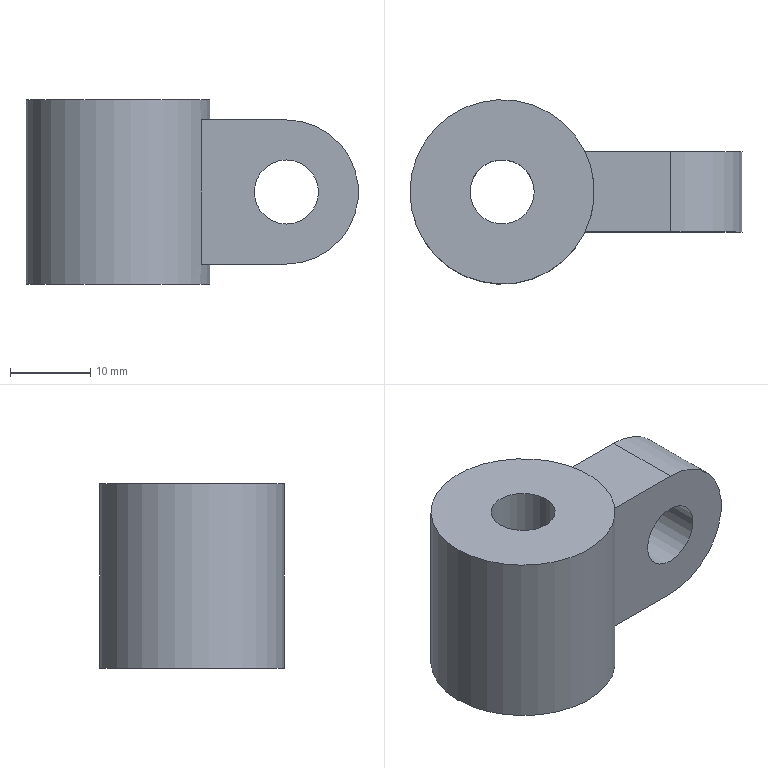Part | STEP file | 1 solid | 10 faces | box 41.5 x 23 x 23 mm | volume 10947 mm3 | plane 6 | cylinder 4 | commonest cylinder face diameters 8 x2 18 x1 23 x1
STEP:
#1=CARTESIAN_POINT('',(0.,0.,0.));
#2=DIRECTION('',(0.,0.,1.));
#3=DIRECTION('',(1.,0.,0.));
#4=AXIS2_PLACEMENT_3D('',#1,#2,#3);
#5=CARTESIAN_POINT('',(-11.5,0.,11.5));
#6=VERTEX_POINT('',#5);
#7=CARTESIAN_POINT('',(0.,0.,11.5));
#8=DIRECTION('',(0.,0.,-1.));
#9=DIRECTION('',(-1.,0.,0.));
#10=AXIS2_PLACEMENT_3D('',#7,#8,#9);
#11=CIRCLE('',#10,11.5);
#12=CARTESIAN_POINT('',(0.,0.,11.5));
#13=DIRECTION('',(0.,0.,-1.));
#14=DIRECTION('',(-1.,0.,0.));
#15=AXIS2_PLACEMENT_3D('',#12,#13,#14);
#16=CYLINDRICAL_SURFACE('',#15,11.5);
#17=CARTESIAN_POINT('',(0.,0.));
#18=DIRECTION('',(1.,0.));
#19=VECTOR('',#18,1.);
#20=LINE('',#17,#19);
#21=(GEOMETRIC_REPRESENTATION_CONTEXT(2)PARAMETRIC_REPRESENTATION_CONTEXT()REPRESENTATION_CONTEXT('',''));
#22=DEFINITIONAL_REPRESENTATION('',(#20),#21);
#23=PCURVE('',#16,#22);
#24=CARTESIAN_POINT('',(0.,0.,11.5));
#25=DIRECTION('',(0.,0.,1.));
#26=DIRECTION('',(1.,0.,0.));
#27=AXIS2_PLACEMENT_3D('',#24,#25,#26);
#28=PLANE('',#27);
#29=CARTESIAN_POINT('',(-11.5,0.));
#30=CARTESIAN_POINT('',(-11.5,19.919));
#31=CARTESIAN_POINT('',(5.75,9.959));
#32=CARTESIAN_POINT('',(23.,0.));
#33=CARTESIAN_POINT('',(5.75,-9.959));
#34=CARTESIAN_POINT('',(-11.5,-19.919));
#35=CARTESIAN_POINT('',(-11.5,0.));
#36=(BOUNDED_CURVE()B_SPLINE_CURVE(2,(#29,#30,#31,#32,#33,#34,#35),.UNSPECIFIED.,.T.,.F.)B_SPLINE_CURVE_WITH_KNOTS((1,2,2,2,2,1),(-2.094,0.,2.094,4.189,6.283,8.378),.UNSPECIFIED.)CURVE()GEOMETRIC_REPRESENTATION_ITEM()RATIONAL_B_SPLINE_CURVE((1.,0.5,1.,0.5,1.,0.5,1.))REPRESENTATION_ITEM(''));
#37=(GEOMETRIC_REPRESENTATION_CONTEXT(2)PARAMETRIC_REPRESENTATION_CONTEXT()REPRESENTATION_CONTEXT('',''));
#38=DEFINITIONAL_REPRESENTATION('',(#36),#37);
#39=PCURVE('',#28,#38);
#40=SURFACE_CURVE('',#11,(#23,#39),.PCURVE_S1.);
#41=EDGE_CURVE('',#6,#6,#40,.T.);
#42=ORIENTED_EDGE('',*,*,#41,.T.);
#43=CARTESIAN_POINT('',(-11.5,0.,-11.5));
#44=VERTEX_POINT('',#43);
#45=CARTESIAN_POINT('',(-11.5,0.,11.5));
#46=CARTESIAN_POINT('',(-11.5,0.,-11.5));
#47=B_SPLINE_CURVE_WITH_KNOTS('',1,(#45,#46),.UNSPECIFIED.,.F.,.F.,(2,2),(0.,23.),.PIECEWISE_BEZIER_KNOTS.);
#48=CARTESIAN_POINT('',(6.283,0.));
#49=DIRECTION('',(0.,1.));
#50=VECTOR('',#49,1.);
#51=LINE('',#48,#50);
#52=(GEOMETRIC_REPRESENTATION_CONTEXT(2)PARAMETRIC_REPRESENTATION_CONTEXT()REPRESENTATION_CONTEXT('',''));
#53=DEFINITIONAL_REPRESENTATION('',(#51),#52);
#54=PCURVE('',#16,#53);
#55=CARTESIAN_POINT('',(0.,0.));
#56=DIRECTION('',(0.,1.));
#57=VECTOR('',#56,1.);
#58=LINE('',#55,#57);
#59=(GEOMETRIC_REPRESENTATION_CONTEXT(2)PARAMETRIC_REPRESENTATION_CONTEXT()REPRESENTATION_CONTEXT('',''));
#60=DEFINITIONAL_REPRESENTATION('',(#58),#59);
#61=PCURVE('',#16,#60);
#62=SEAM_CURVE('',#47,(#54,#61),.PCURVE_S1.);
#63=EDGE_CURVE('',#6,#44,#62,.T.);
#64=ORIENTED_EDGE('',*,*,#63,.T.);
#65=CARTESIAN_POINT('',(0.,0.,-11.5));
#66=DIRECTION('',(0.,0.,1.));
#67=DIRECTION('',(-1.,0.,0.));
#68=AXIS2_PLACEMENT_3D('',#65,#66,#67);
#69=CIRCLE('',#68,11.5);
#70=CARTESIAN_POINT('',(6.283,23.));
#71=DIRECTION('',(-1.,0.));
#72=VECTOR('',#71,1.);
#73=LINE('',#70,#72);
#74=(GEOMETRIC_REPRESENTATION_CONTEXT(2)PARAMETRIC_REPRESENTATION_CONTEXT()REPRESENTATION_CONTEXT('',''));
#75=DEFINITIONAL_REPRESENTATION('',(#73),#74);
#76=PCURVE('',#16,#75);
#77=CARTESIAN_POINT('',(0.,0.,-11.5));
#78=DIRECTION('',(0.,0.,1.));
#79=DIRECTION('',(1.,0.,0.));
#80=AXIS2_PLACEMENT_3D('',#77,#78,#79);
#81=PLANE('',#80);
#82=CARTESIAN_POINT('',(0.,0.));
#83=DIRECTION('',(-1.,0.));
#84=AXIS2_PLACEMENT_2D('',#82,#83);
#85=CIRCLE('',#84,11.5);
#86=(GEOMETRIC_REPRESENTATION_CONTEXT(2)PARAMETRIC_REPRESENTATION_CONTEXT()REPRESENTATION_CONTEXT('',''));
#87=DEFINITIONAL_REPRESENTATION('',(#85),#86);
#88=PCURVE('',#81,#87);
#89=SURFACE_CURVE('',#69,(#76,#88),.PCURVE_S1.);
#90=EDGE_CURVE('',#44,#44,#89,.T.);
#91=ORIENTED_EDGE('',*,*,#90,.T.);
#92=ORIENTED_EDGE('',*,*,#63,.F.);
#93=EDGE_LOOP('',(#42,#64,#91,#92));
#94=FACE_BOUND('',#93,.T.);
#95=CARTESIAN_POINT('',(10.356,-5.,-9.));
#96=VERTEX_POINT('',#95);
#97=CARTESIAN_POINT('',(10.356,-5.,9.));
#98=VERTEX_POINT('',#97);
#99=CARTESIAN_POINT('',(10.356,-5.,11.5));
#100=DIRECTION('',(0.,0.,1.));
#101=VECTOR('',#100,1.);
#102=LINE('',#99,#101);
#103=CARTESIAN_POINT('',(3.591,0.));
#104=DIRECTION('',(0.,-1.));
#105=VECTOR('',#104,1.);
#106=LINE('',#103,#105);
#107=(GEOMETRIC_REPRESENTATION_CONTEXT(2)PARAMETRIC_REPRESENTATION_CONTEXT()REPRESENTATION_CONTEXT('',''));
#108=DEFINITIONAL_REPRESENTATION('',(#106),#107);
#109=PCURVE('',#16,#108);
#110=CARTESIAN_POINT('',(0.,-5.,0.));
#111=DIRECTION('',(0.,1.,0.));
#112=DIRECTION('',(0.,0.,1.));
#113=AXIS2_PLACEMENT_3D('',#110,#111,#112);
#114=PLANE('',#113);
#115=CARTESIAN_POINT('',(11.5,10.356));
#116=DIRECTION('',(1.,0.));
#117=VECTOR('',#116,1.);
#118=LINE('',#115,#117);
#119=(GEOMETRIC_REPRESENTATION_CONTEXT(2)PARAMETRIC_REPRESENTATION_CONTEXT()REPRESENTATION_CONTEXT('',''));
#120=DEFINITIONAL_REPRESENTATION('',(#118),#119);
#121=PCURVE('',#114,#120);
#122=SURFACE_CURVE('',#102,(#109,#121),.PCURVE_S1.);
#123=EDGE_CURVE('',#96,#98,#122,.T.);
#124=ORIENTED_EDGE('',*,*,#123,.T.);
#125=CARTESIAN_POINT('',(10.356,5.,9.));
#126=VERTEX_POINT('',#125);
#127=CARTESIAN_POINT('',(0.,0.,9.));
#128=DIRECTION('',(0.,0.,1.));
#129=DIRECTION('',(-1.,0.,0.));
#130=AXIS2_PLACEMENT_3D('',#127,#128,#129);
#131=CIRCLE('',#130,11.5);
#132=CARTESIAN_POINT('',(6.283,2.5));
#133=DIRECTION('',(-1.,0.));
#134=VECTOR('',#133,1.);
#135=LINE('',#132,#134);
#136=(GEOMETRIC_REPRESENTATION_CONTEXT(2)PARAMETRIC_REPRESENTATION_CONTEXT()REPRESENTATION_CONTEXT('',''));
#137=DEFINITIONAL_REPRESENTATION('',(#135),#136);
#138=PCURVE('',#16,#137);
#139=CARTESIAN_POINT('',(10.,5.,9.));
#140=DIRECTION('',(0.,0.,-1.));
#141=DIRECTION('',(-1.,0.,0.));
#142=AXIS2_PLACEMENT_3D('',#139,#140,#141);
#143=PLANE('',#142);
#144=CARTESIAN_POINT('',(21.5,-5.));
#145=CARTESIAN_POINT('',(21.5,-24.919));
#146=CARTESIAN_POINT('',(4.25,-14.959));
#147=CARTESIAN_POINT('',(-13.,-5.));
#148=CARTESIAN_POINT('',(4.25,4.959));
#149=CARTESIAN_POINT('',(21.5,14.919));
#150=CARTESIAN_POINT('',(21.5,-5.));
#151=(BOUNDED_CURVE()B_SPLINE_CURVE(2,(#144,#145,#146,#147,#148,#149,#150),.UNSPECIFIED.,.T.,.F.)B_SPLINE_CURVE_WITH_KNOTS((1,2,2,2,2,1),(-2.094,0.,2.094,4.189,6.283,8.378),.UNSPECIFIED.)CURVE()GEOMETRIC_REPRESENTATION_ITEM()RATIONAL_B_SPLINE_CURVE((1.,0.5,1.,0.5,1.,0.5,1.))REPRESENTATION_ITEM(''));
#152=(GEOMETRIC_REPRESENTATION_CONTEXT(2)PARAMETRIC_REPRESENTATION_CONTEXT()REPRESENTATION_CONTEXT('',''));
#153=DEFINITIONAL_REPRESENTATION('',(#151),#152);
#154=PCURVE('',#143,#153);
#155=SURFACE_CURVE('',#131,(#138,#154),.PCURVE_S1.);
#156=EDGE_CURVE('',#98,#126,#155,.T.);
#157=ORIENTED_EDGE('',*,*,#156,.T.);
#158=CARTESIAN_POINT('',(10.356,5.,-9.));
#159=VERTEX_POINT('',#158);
#160=CARTESIAN_POINT('',(10.356,5.,11.5));
#161=DIRECTION('',(0.,0.,-1.));
#162=VECTOR('',#161,1.);
#163=LINE('',#160,#162);
#164=CARTESIAN_POINT('',(2.692,0.));
#165=DIRECTION('',(0.,1.));
#166=VECTOR('',#165,1.);
#167=LINE('',#164,#166);
#168=(GEOMETRIC_REPRESENTATION_CONTEXT(2)PARAMETRIC_REPRESENTATION_CONTEXT()REPRESENTATION_CONTEXT('',''));
#169=DEFINITIONAL_REPRESENTATION('',(#167),#168);
#170=PCURVE('',#16,#169);
#171=CARTESIAN_POINT('',(0.,5.,0.));
#172=DIRECTION('',(0.,1.,0.));
#173=DIRECTION('',(0.,0.,1.));
#174=AXIS2_PLACEMENT_3D('',#171,#172,#173);
#175=PLANE('',#174);
#176=CARTESIAN_POINT('',(11.5,10.356));
#177=DIRECTION('',(-1.,0.));
#178=VECTOR('',#177,1.);
#179=LINE('',#176,#178);
#180=(GEOMETRIC_REPRESENTATION_CONTEXT(2)PARAMETRIC_REPRESENTATION_CONTEXT()REPRESENTATION_CONTEXT('',''));
#181=DEFINITIONAL_REPRESENTATION('',(#179),#180);
#182=PCURVE('',#175,#181);
#183=SURFACE_CURVE('',#163,(#170,#182),.PCURVE_S1.);
#184=EDGE_CURVE('',#126,#159,#183,.T.);
#185=ORIENTED_EDGE('',*,*,#184,.T.);
#186=CARTESIAN_POINT('',(0.,0.,-9.));
#187=DIRECTION('',(0.,0.,-1.));
#188=DIRECTION('',(-1.,0.,0.));
#189=AXIS2_PLACEMENT_3D('',#186,#187,#188);
#190=CIRCLE('',#189,11.5);
#191=CARTESIAN_POINT('',(0.,20.5));
#192=DIRECTION('',(1.,0.));
#193=VECTOR('',#192,1.);
#194=LINE('',#191,#193);
#195=(GEOMETRIC_REPRESENTATION_CONTEXT(2)PARAMETRIC_REPRESENTATION_CONTEXT()REPRESENTATION_CONTEXT('',''));
#196=DEFINITIONAL_REPRESENTATION('',(#194),#195);
#197=PCURVE('',#16,#196);
#198=CARTESIAN_POINT('',(10.,5.,-9.));
#199=DIRECTION('',(0.,0.,1.));
#200=DIRECTION('',(1.,0.,0.));
#201=AXIS2_PLACEMENT_3D('',#198,#199,#200);
#202=PLANE('',#201);
#203=CARTESIAN_POINT('',(-21.5,-5.));
#204=CARTESIAN_POINT('',(-21.5,14.919));
#205=CARTESIAN_POINT('',(-4.25,4.959));
#206=CARTESIAN_POINT('',(13.,-5.));
#207=CARTESIAN_POINT('',(-4.25,-14.959));
#208=CARTESIAN_POINT('',(-21.5,-24.919));
#209=CARTESIAN_POINT('',(-21.5,-5.));
#210=(BOUNDED_CURVE()B_SPLINE_CURVE(2,(#203,#204,#205,#206,#207,#208,#209),.UNSPECIFIED.,.T.,.F.)B_SPLINE_CURVE_WITH_KNOTS((1,2,2,2,2,1),(-2.094,0.,2.094,4.189,6.283,8.378),.UNSPECIFIED.)CURVE()GEOMETRIC_REPRESENTATION_ITEM()RATIONAL_B_SPLINE_CURVE((1.,0.5,1.,0.5,1.,0.5,1.))REPRESENTATION_ITEM(''));
#211=(GEOMETRIC_REPRESENTATION_CONTEXT(2)PARAMETRIC_REPRESENTATION_CONTEXT()REPRESENTATION_CONTEXT('',''));
#212=DEFINITIONAL_REPRESENTATION('',(#210),#211);
#213=PCURVE('',#202,#212);
#214=SURFACE_CURVE('',#190,(#197,#213),.PCURVE_S1.);
#215=EDGE_CURVE('',#159,#96,#214,.T.);
#216=ORIENTED_EDGE('',*,*,#215,.T.);
#217=EDGE_LOOP('',(#124,#157,#185,#216));
#218=FACE_BOUND('',#217,.T.);
#219=ADVANCED_FACE('',(#94,#218),#16,.T.);
#220=CARTESIAN_POINT('',(21.,5.,9.));
#221=VERTEX_POINT('',#220);
#222=CARTESIAN_POINT('',(21.,-5.,9.));
#223=VERTEX_POINT('',#222);
#224=CARTESIAN_POINT('',(21.,5.,9.));
#225=DIRECTION('',(0.,-1.,0.));
#226=VECTOR('',#225,1.);
#227=LINE('',#224,#226);
#228=CARTESIAN_POINT('',(-11.,0.));
#229=DIRECTION('',(0.,-1.));
#230=VECTOR('',#229,1.);
#231=LINE('',#228,#230);
#232=(GEOMETRIC_REPRESENTATION_CONTEXT(2)PARAMETRIC_REPRESENTATION_CONTEXT()REPRESENTATION_CONTEXT('',''));
#233=DEFINITIONAL_REPRESENTATION('',(#231),#232);
#234=PCURVE('',#143,#233);
#235=CARTESIAN_POINT('',(21.,5.,0.));
#236=DIRECTION('',(0.,-1.,0.));
#237=DIRECTION('',(0.,0.,-1.));
#238=AXIS2_PLACEMENT_3D('',#235,#236,#237);
#239=CYLINDRICAL_SURFACE('',#238,9.);
#240=CARTESIAN_POINT('',(3.142,0.));
#241=DIRECTION('',(0.,1.));
#242=VECTOR('',#241,1.);
#243=LINE('',#240,#242);
#244=(GEOMETRIC_REPRESENTATION_CONTEXT(2)PARAMETRIC_REPRESENTATION_CONTEXT()REPRESENTATION_CONTEXT('',''));
#245=DEFINITIONAL_REPRESENTATION('',(#243),#244);
#246=PCURVE('',#239,#245);
#247=SURFACE_CURVE('',#227,(#234,#246),.PCURVE_S1.);
#248=EDGE_CURVE('',#221,#223,#247,.T.);
#249=ORIENTED_EDGE('',*,*,#248,.F.);
#250=CARTESIAN_POINT('',(10.,5.,9.));
#251=DIRECTION('',(1.,0.,0.));
#252=VECTOR('',#251,1.);
#253=LINE('',#250,#252);
#254=CARTESIAN_POINT('',(0.,0.));
#255=DIRECTION('',(-1.,0.));
#256=VECTOR('',#255,1.);
#257=LINE('',#254,#256);
#258=(GEOMETRIC_REPRESENTATION_CONTEXT(2)PARAMETRIC_REPRESENTATION_CONTEXT()REPRESENTATION_CONTEXT('',''));
#259=DEFINITIONAL_REPRESENTATION('',(#257),#258);
#260=PCURVE('',#143,#259);
#261=CARTESIAN_POINT('',(9.,10.));
#262=DIRECTION('',(0.,1.));
#263=VECTOR('',#262,1.);
#264=LINE('',#261,#263);
#265=(GEOMETRIC_REPRESENTATION_CONTEXT(2)PARAMETRIC_REPRESENTATION_CONTEXT()REPRESENTATION_CONTEXT('',''));
#266=DEFINITIONAL_REPRESENTATION('',(#264),#265);
#267=PCURVE('',#175,#266);
#268=SURFACE_CURVE('',#253,(#260,#267),.PCURVE_S1.);
#269=EDGE_CURVE('',#126,#221,#268,.T.);
#270=ORIENTED_EDGE('',*,*,#269,.F.);
#271=ORIENTED_EDGE('',*,*,#156,.F.);
#272=CARTESIAN_POINT('',(10.,-5.,9.));
#273=DIRECTION('',(-1.,0.,0.));
#274=VECTOR('',#273,1.);
#275=LINE('',#272,#274);
#276=CARTESIAN_POINT('',(0.,-10.));
#277=DIRECTION('',(1.,0.));
#278=VECTOR('',#277,1.);
#279=LINE('',#276,#278);
#280=(GEOMETRIC_REPRESENTATION_CONTEXT(2)PARAMETRIC_REPRESENTATION_CONTEXT()REPRESENTATION_CONTEXT('',''));
#281=DEFINITIONAL_REPRESENTATION('',(#279),#280);
#282=PCURVE('',#143,#281);
#283=CARTESIAN_POINT('',(9.,10.));
#284=DIRECTION('',(0.,-1.));
#285=VECTOR('',#284,1.);
#286=LINE('',#283,#285);
#287=(GEOMETRIC_REPRESENTATION_CONTEXT(2)PARAMETRIC_REPRESENTATION_CONTEXT()REPRESENTATION_CONTEXT('',''));
#288=DEFINITIONAL_REPRESENTATION('',(#286),#287);
#289=PCURVE('',#114,#288);
#290=SURFACE_CURVE('',#275,(#282,#289),.PCURVE_S1.);
#291=EDGE_CURVE('',#223,#98,#290,.T.);
#292=ORIENTED_EDGE('',*,*,#291,.F.);
#293=EDGE_LOOP('',(#249,#270,#271,#292));
#294=FACE_BOUND('',#293,.T.);
#295=ADVANCED_FACE('',(#294),#143,.F.);
#296=CARTESIAN_POINT('',(21.,-5.,4.));
#297=VERTEX_POINT('',#296);
#298=CARTESIAN_POINT('',(21.,-5.,0.));
#299=DIRECTION('',(0.,-1.,0.));
#300=DIRECTION('',(0.,0.,1.));
#301=AXIS2_PLACEMENT_3D('',#298,#299,#300);
#302=CIRCLE('',#301,4.);
#303=CARTESIAN_POINT('',(4.,21.));
#304=CARTESIAN_POINT('',(4.,14.072));
#305=CARTESIAN_POINT('',(-2.,17.536));
#306=CARTESIAN_POINT('',(-8.,21.));
#307=CARTESIAN_POINT('',(-2.,24.464));
#308=CARTESIAN_POINT('',(4.,27.928));
#309=CARTESIAN_POINT('',(4.,21.));
#310=(BOUNDED_CURVE()B_SPLINE_CURVE(2,(#303,#304,#305,#306,#307,#308,#309),.UNSPECIFIED.,.T.,.F.)B_SPLINE_CURVE_WITH_KNOTS((1,2,2,2,2,1),(-2.094,0.,2.094,4.189,6.283,8.378),.UNSPECIFIED.)CURVE()GEOMETRIC_REPRESENTATION_ITEM()RATIONAL_B_SPLINE_CURVE((1.,0.5,1.,0.5,1.,0.5,1.))REPRESENTATION_ITEM(''));
#311=(GEOMETRIC_REPRESENTATION_CONTEXT(2)PARAMETRIC_REPRESENTATION_CONTEXT()REPRESENTATION_CONTEXT('',''));
#312=DEFINITIONAL_REPRESENTATION('',(#310),#311);
#313=PCURVE('',#114,#312);
#314=CARTESIAN_POINT('',(21.,-5.,0.));
#315=DIRECTION('',(0.,1.,0.));
#316=DIRECTION('',(0.,0.,1.));
#317=AXIS2_PLACEMENT_3D('',#314,#315,#316);
#318=CYLINDRICAL_SURFACE('',#317,4.);
#319=CARTESIAN_POINT('',(6.283,0.));
#320=DIRECTION('',(-1.,0.));
#321=VECTOR('',#320,1.);
#322=LINE('',#319,#321);
#323=(GEOMETRIC_REPRESENTATION_CONTEXT(2)PARAMETRIC_REPRESENTATION_CONTEXT()REPRESENTATION_CONTEXT('',''));
#324=DEFINITIONAL_REPRESENTATION('',(#322),#323);
#325=PCURVE('',#318,#324);
#326=SURFACE_CURVE('',#302,(#313,#325),.PCURVE_S1.);
#327=EDGE_CURVE('',#297,#297,#326,.T.);
#328=ORIENTED_EDGE('',*,*,#327,.F.);
#329=EDGE_LOOP('',(#328));
#330=FACE_BOUND('',#329,.T.);
#331=CARTESIAN_POINT('',(21.,-5.,-9.));
#332=VERTEX_POINT('',#331);
#333=CARTESIAN_POINT('',(21.,-5.,0.));
#334=DIRECTION('',(0.,1.,0.));
#335=DIRECTION('',(0.,0.,-1.));
#336=AXIS2_PLACEMENT_3D('',#333,#334,#335);
#337=CIRCLE('',#336,9.);
#338=CARTESIAN_POINT('',(0.,21.));
#339=DIRECTION('',(-1.,0.));
#340=AXIS2_PLACEMENT_2D('',#338,#339);
#341=CIRCLE('',#340,9.);
#342=(GEOMETRIC_REPRESENTATION_CONTEXT(2)PARAMETRIC_REPRESENTATION_CONTEXT()REPRESENTATION_CONTEXT('',''));
#343=DEFINITIONAL_REPRESENTATION('',(#341),#342);
#344=PCURVE('',#114,#343);
#345=CARTESIAN_POINT('',(6.283,10.));
#346=DIRECTION('',(-1.,0.));
#347=VECTOR('',#346,1.);
#348=LINE('',#345,#347);
#349=(GEOMETRIC_REPRESENTATION_CONTEXT(2)PARAMETRIC_REPRESENTATION_CONTEXT()REPRESENTATION_CONTEXT('',''));
#350=DEFINITIONAL_REPRESENTATION('',(#348),#349);
#351=PCURVE('',#239,#350);
#352=SURFACE_CURVE('',#337,(#344,#351),.PCURVE_S1.);
#353=EDGE_CURVE('',#223,#332,#352,.T.);
#354=ORIENTED_EDGE('',*,*,#353,.F.);
#355=ORIENTED_EDGE('',*,*,#291,.T.);
#356=ORIENTED_EDGE('',*,*,#123,.F.);
#357=CARTESIAN_POINT('',(0.,-5.,-9.));
#358=DIRECTION('',(-1.,0.,0.));
#359=VECTOR('',#358,1.);
#360=LINE('',#357,#359);
#361=CARTESIAN_POINT('',(-9.,0.));
#362=DIRECTION('',(0.,-1.));
#363=VECTOR('',#362,1.);
#364=LINE('',#361,#363);
#365=(GEOMETRIC_REPRESENTATION_CONTEXT(2)PARAMETRIC_REPRESENTATION_CONTEXT()REPRESENTATION_CONTEXT('',''));
#366=DEFINITIONAL_REPRESENTATION('',(#364),#365);
#367=PCURVE('',#114,#366);
#368=CARTESIAN_POINT('',(-10.,-10.));
#369=DIRECTION('',(-1.,0.));
#370=VECTOR('',#369,1.);
#371=LINE('',#368,#370);
#372=(GEOMETRIC_REPRESENTATION_CONTEXT(2)PARAMETRIC_REPRESENTATION_CONTEXT()REPRESENTATION_CONTEXT('',''));
#373=DEFINITIONAL_REPRESENTATION('',(#371),#372);
#374=PCURVE('',#202,#373);
#375=SURFACE_CURVE('',#360,(#367,#374),.PCURVE_S1.);
#376=EDGE_CURVE('',#332,#96,#375,.T.);
#377=ORIENTED_EDGE('',*,*,#376,.F.);
#378=EDGE_LOOP('',(#354,#355,#356,#377));
#379=FACE_BOUND('',#378,.T.);
#380=ADVANCED_FACE('',(#330,#379),#114,.F.);
#381=CARTESIAN_POINT('',(21.,5.,-9.));
#382=VERTEX_POINT('',#381);
#383=CARTESIAN_POINT('',(21.,5.,-9.));
#384=DIRECTION('',(0.,1.,0.));
#385=VECTOR('',#384,1.);
#386=LINE('',#383,#385);
#387=CARTESIAN_POINT('',(11.,0.));
#388=DIRECTION('',(0.,1.));
#389=VECTOR('',#388,1.);
#390=LINE('',#387,#389);
#391=(GEOMETRIC_REPRESENTATION_CONTEXT(2)PARAMETRIC_REPRESENTATION_CONTEXT()REPRESENTATION_CONTEXT('',''));
#392=DEFINITIONAL_REPRESENTATION('',(#390),#391);
#393=PCURVE('',#202,#392);
#394=CARTESIAN_POINT('',(0.,0.));
#395=DIRECTION('',(0.,-1.));
#396=VECTOR('',#395,1.);
#397=LINE('',#394,#396);
#398=(GEOMETRIC_REPRESENTATION_CONTEXT(2)PARAMETRIC_REPRESENTATION_CONTEXT()REPRESENTATION_CONTEXT('',''));
#399=DEFINITIONAL_REPRESENTATION('',(#397),#398);
#400=PCURVE('',#239,#399);
#401=SURFACE_CURVE('',#386,(#393,#400),.PCURVE_S1.);
#402=EDGE_CURVE('',#332,#382,#401,.T.);
#403=ORIENTED_EDGE('',*,*,#402,.F.);
#404=ORIENTED_EDGE('',*,*,#376,.T.);
#405=ORIENTED_EDGE('',*,*,#215,.F.);
#406=CARTESIAN_POINT('',(10.,5.,-9.));
#407=DIRECTION('',(-1.,0.,0.));
#408=VECTOR('',#407,1.);
#409=LINE('',#406,#408);
#410=CARTESIAN_POINT('',(0.,0.));
#411=DIRECTION('',(-1.,0.));
#412=VECTOR('',#411,1.);
#413=LINE('',#410,#412);
#414=(GEOMETRIC_REPRESENTATION_CONTEXT(2)PARAMETRIC_REPRESENTATION_CONTEXT()REPRESENTATION_CONTEXT('',''));
#415=DEFINITIONAL_REPRESENTATION('',(#413),#414);
#416=PCURVE('',#202,#415);
#417=CARTESIAN_POINT('',(-9.,10.));
#418=DIRECTION('',(0.,-1.));
#419=VECTOR('',#418,1.);
#420=LINE('',#417,#419);
#421=(GEOMETRIC_REPRESENTATION_CONTEXT(2)PARAMETRIC_REPRESENTATION_CONTEXT()REPRESENTATION_CONTEXT('',''));
#422=DEFINITIONAL_REPRESENTATION('',(#420),#421);
#423=PCURVE('',#175,#422);
#424=SURFACE_CURVE('',#409,(#416,#423),.PCURVE_S1.);
#425=EDGE_CURVE('',#382,#159,#424,.T.);
#426=ORIENTED_EDGE('',*,*,#425,.F.);
#427=EDGE_LOOP('',(#403,#404,#405,#426));
#428=FACE_BOUND('',#427,.T.);
#429=ADVANCED_FACE('',(#428),#202,.F.);
#430=CARTESIAN_POINT('',(-4.,0.,-11.5));
#431=VERTEX_POINT('',#430);
#432=CARTESIAN_POINT('',(0.,0.,-11.5));
#433=DIRECTION('',(0.,0.,-1.));
#434=DIRECTION('',(-1.,0.,0.));
#435=AXIS2_PLACEMENT_3D('',#432,#433,#434);
#436=CIRCLE('',#435,4.);
#437=CARTESIAN_POINT('',(-4.,0.));
#438=CARTESIAN_POINT('',(-4.,6.928));
#439=CARTESIAN_POINT('',(2.,3.464));
#440=CARTESIAN_POINT('',(8.,0.));
#441=CARTESIAN_POINT('',(2.,-3.464));
#442=CARTESIAN_POINT('',(-4.,-6.928));
#443=CARTESIAN_POINT('',(-4.,0.));
#444=(BOUNDED_CURVE()B_SPLINE_CURVE(2,(#437,#438,#439,#440,#441,#442,#443),.UNSPECIFIED.,.T.,.F.)B_SPLINE_CURVE_WITH_KNOTS((1,2,2,2,2,1),(-2.094,0.,2.094,4.189,6.283,8.378),.UNSPECIFIED.)CURVE()GEOMETRIC_REPRESENTATION_ITEM()RATIONAL_B_SPLINE_CURVE((1.,0.5,1.,0.5,1.,0.5,1.))REPRESENTATION_ITEM(''));
#445=(GEOMETRIC_REPRESENTATION_CONTEXT(2)PARAMETRIC_REPRESENTATION_CONTEXT()REPRESENTATION_CONTEXT('',''));
#446=DEFINITIONAL_REPRESENTATION('',(#444),#445);
#447=PCURVE('',#81,#446);
#448=CARTESIAN_POINT('',(0.,0.,11.5));
#449=DIRECTION('',(0.,0.,-1.));
#450=DIRECTION('',(-1.,0.,0.));
#451=AXIS2_PLACEMENT_3D('',#448,#449,#450);
#452=CYLINDRICAL_SURFACE('',#451,4.);
#453=CARTESIAN_POINT('',(0.,23.));
#454=DIRECTION('',(1.,0.));
#455=VECTOR('',#454,1.);
#456=LINE('',#453,#455);
#457=(GEOMETRIC_REPRESENTATION_CONTEXT(2)PARAMETRIC_REPRESENTATION_CONTEXT()REPRESENTATION_CONTEXT('',''));
#458=DEFINITIONAL_REPRESENTATION('',(#456),#457);
#459=PCURVE('',#452,#458);
#460=SURFACE_CURVE('',#436,(#447,#459),.PCURVE_S1.);
#461=EDGE_CURVE('',#431,#431,#460,.T.);
#462=ORIENTED_EDGE('',*,*,#461,.F.);
#463=EDGE_LOOP('',(#462));
#464=FACE_BOUND('',#463,.T.);
#465=ORIENTED_EDGE('',*,*,#90,.F.);
#466=EDGE_LOOP('',(#465));
#467=FACE_BOUND('',#466,.T.);
#468=ADVANCED_FACE('',(#464,#467),#81,.F.);
#469=CARTESIAN_POINT('',(-4.,0.,11.5));
#470=VERTEX_POINT('',#469);
#471=CARTESIAN_POINT('',(0.,0.,11.5));
#472=DIRECTION('',(0.,0.,-1.));
#473=DIRECTION('',(-1.,0.,0.));
#474=AXIS2_PLACEMENT_3D('',#471,#472,#473);
#475=CIRCLE('',#474,4.);
#476=CARTESIAN_POINT('',(-4.,0.));
#477=CARTESIAN_POINT('',(-4.,6.928));
#478=CARTESIAN_POINT('',(2.,3.464));
#479=CARTESIAN_POINT('',(8.,0.));
#480=CARTESIAN_POINT('',(2.,-3.464));
#481=CARTESIAN_POINT('',(-4.,-6.928));
#482=CARTESIAN_POINT('',(-4.,0.));
#483=(BOUNDED_CURVE()B_SPLINE_CURVE(2,(#476,#477,#478,#479,#480,#481,#482),.UNSPECIFIED.,.T.,.F.)B_SPLINE_CURVE_WITH_KNOTS((1,2,2,2,2,1),(-2.094,0.,2.094,4.189,6.283,8.378),.UNSPECIFIED.)CURVE()GEOMETRIC_REPRESENTATION_ITEM()RATIONAL_B_SPLINE_CURVE((1.,0.5,1.,0.5,1.,0.5,1.))REPRESENTATION_ITEM(''));
#484=(GEOMETRIC_REPRESENTATION_CONTEXT(2)PARAMETRIC_REPRESENTATION_CONTEXT()REPRESENTATION_CONTEXT('',''));
#485=DEFINITIONAL_REPRESENTATION('',(#483),#484);
#486=PCURVE('',#28,#485);
#487=CARTESIAN_POINT('',(0.,0.));
#488=DIRECTION('',(1.,0.));
#489=VECTOR('',#488,1.);
#490=LINE('',#487,#489);
#491=(GEOMETRIC_REPRESENTATION_CONTEXT(2)PARAMETRIC_REPRESENTATION_CONTEXT()REPRESENTATION_CONTEXT('',''));
#492=DEFINITIONAL_REPRESENTATION('',(#490),#491);
#493=PCURVE('',#452,#492);
#494=SURFACE_CURVE('',#475,(#486,#493),.PCURVE_S1.);
#495=EDGE_CURVE('',#470,#470,#494,.T.);
#496=ORIENTED_EDGE('',*,*,#495,.T.);
#497=EDGE_LOOP('',(#496));
#498=FACE_BOUND('',#497,.T.);
#499=ORIENTED_EDGE('',*,*,#41,.F.);
#500=EDGE_LOOP('',(#499));
#501=FACE_BOUND('',#500,.T.);
#502=ADVANCED_FACE('',(#498,#501),#28,.T.);
#503=ORIENTED_EDGE('',*,*,#248,.T.);
#504=ORIENTED_EDGE('',*,*,#353,.T.);
#505=ORIENTED_EDGE('',*,*,#402,.T.);
#506=CARTESIAN_POINT('',(21.,5.,0.));
#507=DIRECTION('',(0.,-1.,0.));
#508=DIRECTION('',(0.,0.,-1.));
#509=AXIS2_PLACEMENT_3D('',#506,#507,#508);
#510=CIRCLE('',#509,9.);
#511=CARTESIAN_POINT('',(0.,0.));
#512=DIRECTION('',(1.,0.));
#513=VECTOR('',#512,1.);
#514=LINE('',#511,#513);
#515=(GEOMETRIC_REPRESENTATION_CONTEXT(2)PARAMETRIC_REPRESENTATION_CONTEXT()REPRESENTATION_CONTEXT('',''));
#516=DEFINITIONAL_REPRESENTATION('',(#514),#515);
#517=PCURVE('',#239,#516);
#518=CARTESIAN_POINT('',(-9.,21.));
#519=CARTESIAN_POINT('',(-9.,36.588));
#520=CARTESIAN_POINT('',(4.5,28.794));
#521=CARTESIAN_POINT('',(18.,21.));
#522=CARTESIAN_POINT('',(4.5,13.206));
#523=CARTESIAN_POINT('',(-9.,5.412));
#524=CARTESIAN_POINT('',(-9.,21.));
#525=(BOUNDED_CURVE()B_SPLINE_CURVE(2,(#518,#519,#520,#521,#522,#523,#524),.UNSPECIFIED.,.T.,.F.)B_SPLINE_CURVE_WITH_KNOTS((1,2,2,2,2,1),(-2.094,0.,2.094,4.189,6.283,8.378),.UNSPECIFIED.)CURVE()GEOMETRIC_REPRESENTATION_ITEM()RATIONAL_B_SPLINE_CURVE((1.,0.5,1.,0.5,1.,0.5,1.))REPRESENTATION_ITEM(''));
#526=(GEOMETRIC_REPRESENTATION_CONTEXT(2)PARAMETRIC_REPRESENTATION_CONTEXT()REPRESENTATION_CONTEXT('',''));
#527=DEFINITIONAL_REPRESENTATION('',(#525),#526);
#528=PCURVE('',#175,#527);
#529=SURFACE_CURVE('',#510,(#517,#528),.PCURVE_S1.);
#530=EDGE_CURVE('',#382,#221,#529,.T.);
#531=ORIENTED_EDGE('',*,*,#530,.T.);
#532=EDGE_LOOP('',(#503,#504,#505,#531));
#533=FACE_BOUND('',#532,.T.);
#534=ADVANCED_FACE('',(#533),#239,.T.);
#535=CARTESIAN_POINT('',(21.,5.,4.));
#536=VERTEX_POINT('',#535);
#537=CARTESIAN_POINT('',(21.,5.,0.));
#538=DIRECTION('',(0.,-1.,0.));
#539=DIRECTION('',(0.,0.,1.));
#540=AXIS2_PLACEMENT_3D('',#537,#538,#539);
#541=CIRCLE('',#540,4.);
#542=CARTESIAN_POINT('',(4.,21.));
#543=CARTESIAN_POINT('',(4.,14.072));
#544=CARTESIAN_POINT('',(-2.,17.536));
#545=CARTESIAN_POINT('',(-8.,21.));
#546=CARTESIAN_POINT('',(-2.,24.464));
#547=CARTESIAN_POINT('',(4.,27.928));
#548=CARTESIAN_POINT('',(4.,21.));
#549=(BOUNDED_CURVE()B_SPLINE_CURVE(2,(#542,#543,#544,#545,#546,#547,#548),.UNSPECIFIED.,.T.,.F.)B_SPLINE_CURVE_WITH_KNOTS((1,2,2,2,2,1),(-2.094,0.,2.094,4.189,6.283,8.378),.UNSPECIFIED.)CURVE()GEOMETRIC_REPRESENTATION_ITEM()RATIONAL_B_SPLINE_CURVE((1.,0.5,1.,0.5,1.,0.5,1.))REPRESENTATION_ITEM(''));
#550=(GEOMETRIC_REPRESENTATION_CONTEXT(2)PARAMETRIC_REPRESENTATION_CONTEXT()REPRESENTATION_CONTEXT('',''));
#551=DEFINITIONAL_REPRESENTATION('',(#549),#550);
#552=PCURVE('',#175,#551);
#553=CARTESIAN_POINT('',(6.283,10.));
#554=DIRECTION('',(-1.,0.));
#555=VECTOR('',#554,1.);
#556=LINE('',#553,#555);
#557=(GEOMETRIC_REPRESENTATION_CONTEXT(2)PARAMETRIC_REPRESENTATION_CONTEXT()REPRESENTATION_CONTEXT('',''));
#558=DEFINITIONAL_REPRESENTATION('',(#556),#557);
#559=PCURVE('',#318,#558);
#560=SURFACE_CURVE('',#541,(#552,#559),.PCURVE_S1.);
#561=EDGE_CURVE('',#536,#536,#560,.T.);
#562=ORIENTED_EDGE('',*,*,#561,.T.);
#563=EDGE_LOOP('',(#562));
#564=FACE_BOUND('',#563,.T.);
#565=ORIENTED_EDGE('',*,*,#184,.F.);
#566=ORIENTED_EDGE('',*,*,#269,.T.);
#567=ORIENTED_EDGE('',*,*,#530,.F.);
#568=ORIENTED_EDGE('',*,*,#425,.T.);
#569=EDGE_LOOP('',(#565,#566,#567,#568));
#570=FACE_BOUND('',#569,.T.);
#571=ADVANCED_FACE('',(#564,#570),#175,.T.);
#572=ORIENTED_EDGE('',*,*,#327,.F.);
#573=CARTESIAN_POINT('',(21.,-5.,4.));
#574=CARTESIAN_POINT('',(21.,5.,4.));
#575=B_SPLINE_CURVE_WITH_KNOTS('',1,(#573,#574),.UNSPECIFIED.,.F.,.F.,(2,2),(0.,10.),.PIECEWISE_BEZIER_KNOTS.);
#576=CARTESIAN_POINT('',(6.283,0.));
#577=DIRECTION('',(0.,1.));
#578=VECTOR('',#577,1.);
#579=LINE('',#576,#578);
#580=(GEOMETRIC_REPRESENTATION_CONTEXT(2)PARAMETRIC_REPRESENTATION_CONTEXT()REPRESENTATION_CONTEXT('',''));
#581=DEFINITIONAL_REPRESENTATION('',(#579),#580);
#582=PCURVE('',#318,#581);
#583=CARTESIAN_POINT('',(0.,0.));
#584=DIRECTION('',(0.,1.));
#585=VECTOR('',#584,1.);
#586=LINE('',#583,#585);
#587=(GEOMETRIC_REPRESENTATION_CONTEXT(2)PARAMETRIC_REPRESENTATION_CONTEXT()REPRESENTATION_CONTEXT('',''));
#588=DEFINITIONAL_REPRESENTATION('',(#586),#587);
#589=PCURVE('',#318,#588);
#590=SEAM_CURVE('',#575,(#582,#589),.PCURVE_S1.);
#591=EDGE_CURVE('',#297,#536,#590,.T.);
#592=ORIENTED_EDGE('',*,*,#591,.T.);
#593=ORIENTED_EDGE('',*,*,#561,.T.);
#594=ORIENTED_EDGE('',*,*,#591,.F.);
#595=EDGE_LOOP('',(#572,#592,#593,#594));
#596=FACE_BOUND('',#595,.F.);
#597=ADVANCED_FACE('',(#596),#318,.F.);
#598=ORIENTED_EDGE('',*,*,#461,.F.);
#599=CARTESIAN_POINT('',(-4.,0.,11.5));
#600=CARTESIAN_POINT('',(-4.,0.,-11.5));
#601=B_SPLINE_CURVE_WITH_KNOTS('',1,(#599,#600),.UNSPECIFIED.,.F.,.F.,(2,2),(0.,23.),.PIECEWISE_BEZIER_KNOTS.);
#602=CARTESIAN_POINT('',(0.,0.));
#603=DIRECTION('',(0.,1.));
#604=VECTOR('',#603,1.);
#605=LINE('',#602,#604);
#606=(GEOMETRIC_REPRESENTATION_CONTEXT(2)PARAMETRIC_REPRESENTATION_CONTEXT()REPRESENTATION_CONTEXT('',''));
#607=DEFINITIONAL_REPRESENTATION('',(#605),#606);
#608=PCURVE('',#452,#607);
#609=CARTESIAN_POINT('',(6.283,0.));
#610=DIRECTION('',(0.,1.));
#611=VECTOR('',#610,1.);
#612=LINE('',#609,#611);
#613=(GEOMETRIC_REPRESENTATION_CONTEXT(2)PARAMETRIC_REPRESENTATION_CONTEXT()REPRESENTATION_CONTEXT('',''));
#614=DEFINITIONAL_REPRESENTATION('',(#612),#613);
#615=PCURVE('',#452,#614);
#616=SEAM_CURVE('',#601,(#608,#615),.PCURVE_S1.);
#617=EDGE_CURVE('',#470,#431,#616,.T.);
#618=ORIENTED_EDGE('',*,*,#617,.F.);
#619=ORIENTED_EDGE('',*,*,#495,.T.);
#620=ORIENTED_EDGE('',*,*,#617,.T.);
#621=EDGE_LOOP('',(#598,#618,#619,#620));
#622=FACE_BOUND('',#621,.F.);
#623=ADVANCED_FACE('',(#622),#452,.F.);
#624=CLOSED_SHELL('',(#219,#295,#380,#429,#468,#502,#534,#571,#597,#623));
#625=MANIFOLD_SOLID_BREP('',#624);
#626=(LENGTH_UNIT()NAMED_UNIT(*)SI_UNIT(.MILLI.,.METRE.));
#627=UNCERTAINTY_MEASURE_WITH_UNIT(LENGTH_MEASURE(0.000002),#626,'','');
#628=(NAMED_UNIT(*)PLANE_ANGLE_UNIT()SI_UNIT($,.RADIAN.));
#629=(NAMED_UNIT(*)SI_UNIT($,.STERADIAN.)SOLID_ANGLE_UNIT());
#630=(GEOMETRIC_REPRESENTATION_CONTEXT(3)GLOBAL_UNCERTAINTY_ASSIGNED_CONTEXT((#627))GLOBAL_UNIT_ASSIGNED_CONTEXT((#626,#628,#629))REPRESENTATION_CONTEXT('',''));
#631=ADVANCED_BREP_SHAPE_REPRESENTATION('',(#4,#625),#630);